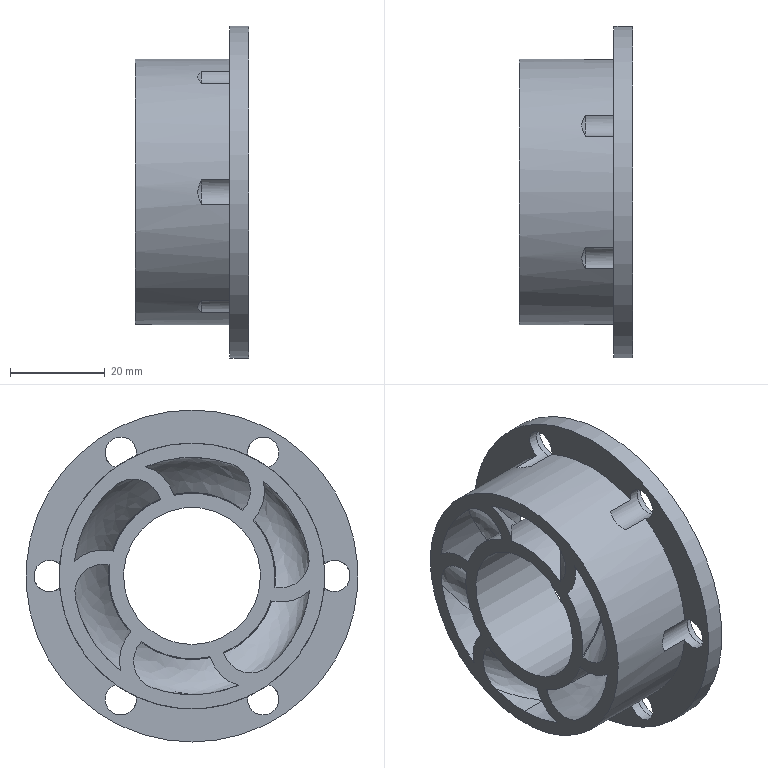Part | STEP file | Swirl | 1 solid | 63 faces | box 24 x 70.2 x 70.2 mm | volume 25661 mm3 | spline 24 | cylinder 23 | plane 10 | cone 6 | commonest cylinder face diameters 6.647 x6 9 x6 35 x6 50.2 x2 29 x1 56.2 x1